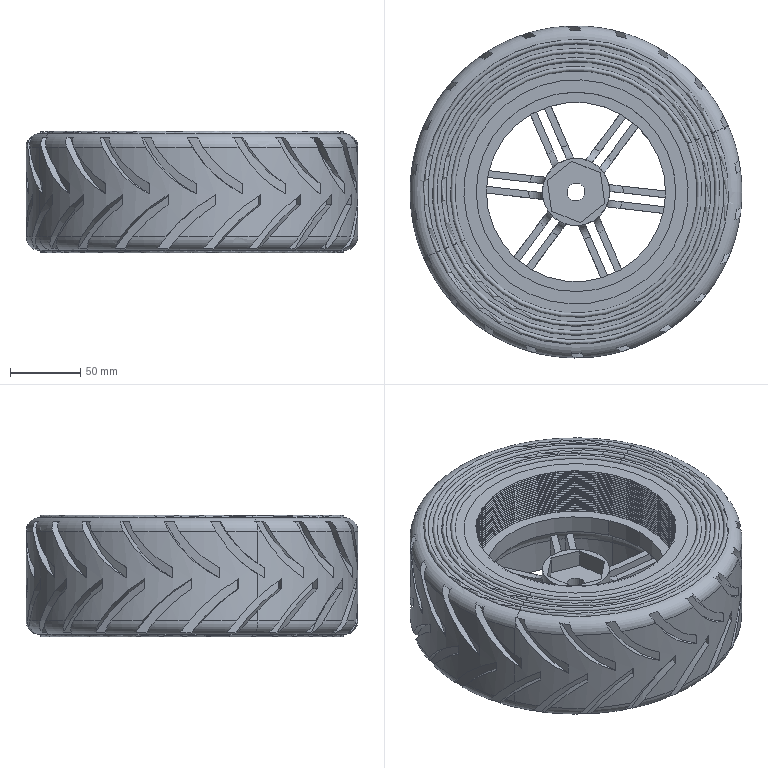Part | SolidWorks | features BaseBody 1 | 1 solid | 470 faces | box 236.8 x 236.8 x 86.4 mm | volume 2369634 mm3 | plane 166 | spline 88 | cone 88 | cylinder 78 | torus 50 | commonest cylinder face diameters 142.4 x46 3.2 x10 8 x10 236.8 x6 12.8 x2 48 x2